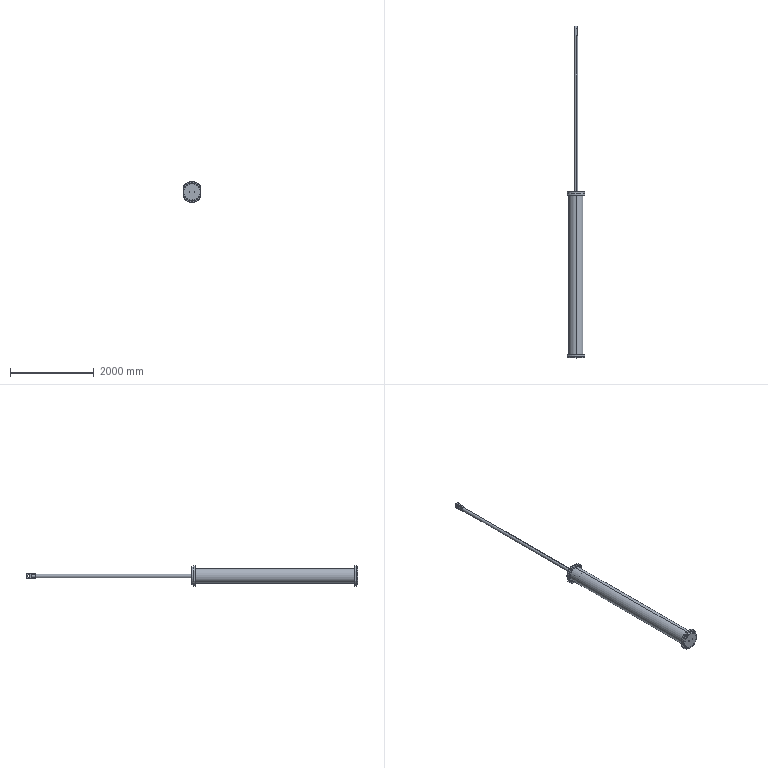Part | SolidWorks | 5 solids | 293 faces | box 430 x 7940 x 500 mm | volume 118465074 mm3 | cylinder 259 | plane 34 | commonest cylinder face diameters 16 x224 60 x6 500 x6 19 x4 80 x4 320 x4